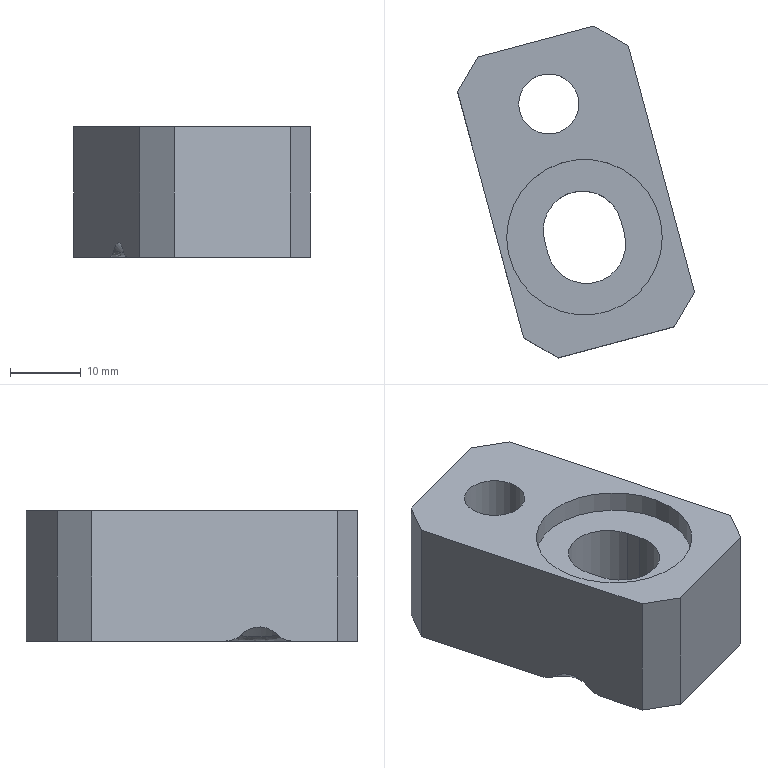Part | NX | features solid 2 | 1 solid | 21 faces | box 33.466 x 46.901 x 18.4 mm | volume 14639 mm3 | plane 14 | cylinder 6 | spline 1 | commonest cylinder face diameters 11.15 x2 8.5 x1 10 x1 14 x1 22 x1
STEP:
#1=CARTESIAN_POINT('',(1426.059,51.189,5.));
#2=VERTEX_POINT('',#1);
#3=CARTESIAN_POINT('',(1421.809,51.189,5.));
#4=DIRECTION('',(0.,0.,1.));
#5=DIRECTION('',(1.,0.,0.));
#6=AXIS2_PLACEMENT_3D('',#3,#4,#5);
#7=CIRCLE('',#6,4.25);
#8=EDGE_CURVE('',#2,#2,#7,.T.);
#9=ORIENTED_EDGE('',*,*,#8,.F.);
#10=EDGE_LOOP('',(#9));
#11=FACE_BOUND('',#10,.T.);
#12=CARTESIAN_POINT('',(1408.924,52.912,5.));
#13=VERTEX_POINT('',#12);
#14=CARTESIAN_POINT('',(1418.241,18.139,5.));
#15=VERTEX_POINT('',#14);
#16=CARTESIAN_POINT('',(1407.889,56.776,5.));
#17=DIRECTION('',(0.2588,-0.9659,0.));
#18=VECTOR('',#17,1000.);
#19=LINE('',#16,#18);
#20=EDGE_CURVE('',#13,#15,#19,.T.);
#21=ORIENTED_EDGE('',*,*,#20,.T.);
#22=CARTESIAN_POINT('',(1423.14,15.311,5.));
#23=VERTEX_POINT('',#22);
#24=CARTESIAN_POINT('',(362.415,627.721,5.));
#25=DIRECTION('',(0.866,-0.5,0.));
#26=VECTOR('',#25,1000.);
#27=LINE('',#24,#26);
#28=EDGE_CURVE('',#15,#23,#27,.T.);
#29=ORIENTED_EDGE('',*,*,#28,.T.);
#30=CARTESIAN_POINT('',(1439.561,19.711,5.));
#31=VERTEX_POINT('',#30);
#32=CARTESIAN_POINT('',(1419.277,14.275,5.));
#33=DIRECTION('',(0.9659,0.2588,0.));
#34=VECTOR('',#33,1000.);
#35=LINE('',#32,#34);
#36=EDGE_CURVE('',#23,#31,#35,.T.);
#37=ORIENTED_EDGE('',*,*,#36,.T.);
#38=CARTESIAN_POINT('',(1442.39,24.61,5.));
#39=VERTEX_POINT('',#38);
#40=CARTESIAN_POINT('',(1071.136,-618.421,5.));
#41=DIRECTION('',(0.5,0.866,0.));
#42=VECTOR('',#41,1000.);
#43=LINE('',#40,#42);
#44=EDGE_CURVE('',#31,#39,#43,.T.);
#45=ORIENTED_EDGE('',*,*,#44,.T.);
#46=CARTESIAN_POINT('',(1433.072,59.383,5.));
#47=VERTEX_POINT('',#46);
#48=CARTESIAN_POINT('',(1443.425,20.746,5.));
#49=DIRECTION('',(-0.2588,0.9659,0.));
#50=VECTOR('',#49,1000.);
#51=LINE('',#48,#50);
#52=EDGE_CURVE('',#39,#47,#51,.T.);
#53=ORIENTED_EDGE('',*,*,#52,.T.);
#54=CARTESIAN_POINT('',(1428.173,62.211,5.));
#55=VERTEX_POINT('',#54);
#56=CARTESIAN_POINT('',(383.982,665.076,5.));
#57=DIRECTION('',(0.866,-0.5,0.));
#58=VECTOR('',#57,1000.);
#59=LINE('',#56,#58);
#60=EDGE_CURVE('',#47,#55,#59,.F.);
#61=ORIENTED_EDGE('',*,*,#60,.T.);
#62=CARTESIAN_POINT('',(1411.752,57.811,5.));
#63=VERTEX_POINT('',#62);
#64=CARTESIAN_POINT('',(1432.037,63.247,5.));
#65=DIRECTION('',(-0.9659,-0.2588,0.));
#66=VECTOR('',#65,1000.);
#67=LINE('',#64,#66);
#68=EDGE_CURVE('',#55,#63,#67,.T.);
#69=ORIENTED_EDGE('',*,*,#68,.T.);
#70=CARTESIAN_POINT('',(1033.781,-596.854,5.));
#71=DIRECTION('',(0.5,0.866,0.));
#72=VECTOR('',#71,1000.);
#73=LINE('',#70,#72);
#74=EDGE_CURVE('',#63,#13,#73,.F.);
#75=ORIENTED_EDGE('',*,*,#74,.T.);
#76=EDGE_LOOP('',(#21,#29,#37,#45,#53,#61,#69,#75));
#77=FACE_BOUND('',#76,.T.);
#78=CARTESIAN_POINT('',(1437.856,32.353,5.));
#79=VERTEX_POINT('',#78);
#80=CARTESIAN_POINT('',(1426.856,32.353,5.));
#81=DIRECTION('',(0.,0.,1.));
#82=DIRECTION('',(1.,0.,0.));
#83=AXIS2_PLACEMENT_3D('',#80,#81,#82);
#84=CIRCLE('',#83,11.);
#85=EDGE_CURVE('',#79,#79,#84,.F.);
#86=ORIENTED_EDGE('',*,*,#85,.T.);
#87=EDGE_LOOP('',(#86));
#88=FACE_BOUND('',#87,.T.);
#89=CARTESIAN_POINT('',(0.,0.,5.));
#90=DIRECTION('',(0.,0.,1.));
#91=DIRECTION('',(1.,0.,0.));
#92=AXIS2_PLACEMENT_3D('',#89,#90,#91);
#93=PLANE('',#92);
#94=ADVANCED_FACE('',(#11,#77,#88),#93,.T.);
#95=ORIENTED_EDGE('',*,*,#85,.F.);
#96=EDGE_LOOP('',(#95));
#97=FACE_BOUND('',#96,.T.);
#98=CARTESIAN_POINT('',(1415.856,32.353,2.));
#99=VERTEX_POINT('',#98);
#100=CARTESIAN_POINT('',(1426.856,32.353,2.));
#101=DIRECTION('',(0.,0.,1.));
#102=DIRECTION('',(-1.,0.,0.));
#103=AXIS2_PLACEMENT_3D('',#100,#101,#102);
#104=CIRCLE('',#103,11.);
#105=EDGE_CURVE('',#99,#99,#104,.T.);
#106=ORIENTED_EDGE('',*,*,#105,.F.);
#107=EDGE_LOOP('',(#106));
#108=FACE_BOUND('',#107,.T.);
#109=CARTESIAN_POINT('',(1426.856,32.353,258.));
#110=DIRECTION('',(0.,0.,-1.));
#111=DIRECTION('',(-1.,0.,0.));
#112=AXIS2_PLACEMENT_3D('',#109,#110,#111);
#113=CYLINDRICAL_SURFACE('',#112,11.);
#114=ADVANCED_FACE('',(#97,#108),#113,.F.);
#115=CARTESIAN_POINT('',(1431.982,34.762,2.));
#116=VERTEX_POINT('',#115);
#117=CARTESIAN_POINT('',(1431.982,34.762,-13.4));
#118=VERTEX_POINT('',#117);
#119=CARTESIAN_POINT('',(1431.982,34.762,-16.4));
#120=DIRECTION('',(0.,0.,1.));
#121=VECTOR('',#120,1000.);
#122=LINE('',#119,#121);
#123=EDGE_CURVE('',#116,#118,#122,.F.);
#124=ORIENTED_EDGE('',*,*,#123,.T.);
#125=CARTESIAN_POINT('',(1432.5,32.83,-13.4));
#126=VERTEX_POINT('',#125);
#127=CARTESIAN_POINT('',(1429.265,44.904,-13.4));
#128=DIRECTION('',(-0.2588,0.9659,0.));
#129=VECTOR('',#128,1000.);
#130=LINE('',#127,#129);
#131=EDGE_CURVE('',#118,#126,#130,.F.);
#132=ORIENTED_EDGE('',*,*,#131,.T.);
#133=CARTESIAN_POINT('',(1432.5,32.83,2.));
#134=VERTEX_POINT('',#133);
#135=CARTESIAN_POINT('',(1432.5,32.83,-16.4));
#136=DIRECTION('',(0.,0.,1.));
#137=VECTOR('',#136,1000.);
#138=LINE('',#135,#137);
#139=EDGE_CURVE('',#134,#126,#138,.F.);
#140=ORIENTED_EDGE('',*,*,#139,.F.);
#141=CARTESIAN_POINT('',(1429.265,44.904,2.));
#142=DIRECTION('',(-0.2588,0.9659,0.));
#143=VECTOR('',#142,1000.);
#144=LINE('',#141,#143);
#145=EDGE_CURVE('',#116,#134,#144,.F.);
#146=ORIENTED_EDGE('',*,*,#145,.F.);
#147=EDGE_LOOP('',(#124,#132,#140,#146));
#148=FACE_BOUND('',#147,.T.);
#149=CARTESIAN_POINT('',(1429.265,44.904,-16.4));
#150=DIRECTION('',(-0.9659,-0.2588,0.));
#151=DIRECTION('',(0.2588,-0.9659,0.));
#152=AXIS2_PLACEMENT_3D('',#149,#150,#151);
#153=PLANE('',#152);
#154=ADVANCED_FACE('',(#148),#153,.T.);
#155=ORIENTED_EDGE('',*,*,#139,.T.);
#156=CARTESIAN_POINT('',(1421.73,29.944,-13.4));
#157=VERTEX_POINT('',#156);
#158=CARTESIAN_POINT('',(1427.115,31.387,-13.4));
#159=DIRECTION('',(0.,0.,1.));
#160=DIRECTION('',(1.,0.,0.));
#161=AXIS2_PLACEMENT_3D('',#158,#159,#160);
#162=CIRCLE('',#161,5.575);
#163=EDGE_CURVE('',#126,#157,#162,.F.);
#164=ORIENTED_EDGE('',*,*,#163,.T.);
#165=CARTESIAN_POINT('',(1421.73,29.944,2.));
#166=VERTEX_POINT('',#165);
#167=CARTESIAN_POINT('',(1421.73,29.944,-16.4));
#168=DIRECTION('',(0.,0.,1.));
#169=VECTOR('',#168,1000.);
#170=LINE('',#167,#169);
#171=EDGE_CURVE('',#166,#157,#170,.F.);
#172=ORIENTED_EDGE('',*,*,#171,.F.);
#173=CARTESIAN_POINT('',(1427.115,31.387,2.));
#174=DIRECTION('',(0.,0.,1.));
#175=DIRECTION('',(-1.,0.,0.));
#176=AXIS2_PLACEMENT_3D('',#173,#174,#175);
#177=CIRCLE('',#176,5.575);
#178=EDGE_CURVE('',#166,#134,#177,.T.);
#179=ORIENTED_EDGE('',*,*,#178,.T.);
#180=EDGE_LOOP('',(#155,#164,#172,#179));
#181=FACE_BOUND('',#180,.T.);
#182=CARTESIAN_POINT('',(1427.115,31.387,-16.4));
#183=DIRECTION('',(0.,0.,1.));
#184=DIRECTION('',(1.,0.,0.));
#185=AXIS2_PLACEMENT_3D('',#182,#183,#184);
#186=CYLINDRICAL_SURFACE('',#185,5.575);
#187=ADVANCED_FACE('',(#181),#186,.F.);
#188=ORIENTED_EDGE('',*,*,#171,.T.);
#189=CARTESIAN_POINT('',(1421.212,31.876,-13.4));
#190=VERTEX_POINT('',#189);
#191=CARTESIAN_POINT('',(1418.495,42.018,-13.4));
#192=DIRECTION('',(0.2588,-0.9659,0.));
#193=VECTOR('',#192,1000.);
#194=LINE('',#191,#193);
#195=EDGE_CURVE('',#157,#190,#194,.F.);
#196=ORIENTED_EDGE('',*,*,#195,.T.);
#197=CARTESIAN_POINT('',(1421.212,31.876,2.));
#198=VERTEX_POINT('',#197);
#199=CARTESIAN_POINT('',(1421.212,31.876,-16.4));
#200=DIRECTION('',(0.,0.,1.));
#201=VECTOR('',#200,1000.);
#202=LINE('',#199,#201);
#203=EDGE_CURVE('',#198,#190,#202,.F.);
#204=ORIENTED_EDGE('',*,*,#203,.F.);
#205=CARTESIAN_POINT('',(1418.495,42.018,2.));
#206=DIRECTION('',(0.2588,-0.9659,0.));
#207=VECTOR('',#206,1000.);
#208=LINE('',#205,#207);
#209=EDGE_CURVE('',#166,#198,#208,.F.);
#210=ORIENTED_EDGE('',*,*,#209,.F.);
#211=EDGE_LOOP('',(#188,#196,#204,#210));
#212=FACE_BOUND('',#211,.T.);
#213=CARTESIAN_POINT('',(1418.495,42.018,-16.4));
#214=DIRECTION('',(0.9659,0.2588,0.));
#215=DIRECTION('',(-0.2588,0.9659,0.));
#216=AXIS2_PLACEMENT_3D('',#213,#214,#215);
#217=PLANE('',#216);
#218=ADVANCED_FACE('',(#212),#217,.T.);
#219=CARTESIAN_POINT('',(1433.072,59.383,-13.4));
#220=VERTEX_POINT('',#219);
#221=CARTESIAN_POINT('',(1442.39,24.61,-13.4));
#222=VERTEX_POINT('',#221);
#223=CARTESIAN_POINT('',(1436.437,46.826,-13.4));
#224=DIRECTION('',(-0.2588,0.9659,0.));
#225=VECTOR('',#224,1000.);
#226=LINE('',#223,#225);
#227=EDGE_CURVE('',#220,#222,#226,.F.);
#228=ORIENTED_EDGE('',*,*,#227,.F.);
#229=CARTESIAN_POINT('',(1433.072,59.383,-16.4));
#230=DIRECTION('',(0.,0.,-1.));
#231=VECTOR('',#230,1000.);
#232=LINE('',#229,#231);
#233=EDGE_CURVE('',#220,#47,#232,.F.);
#234=ORIENTED_EDGE('',*,*,#233,.T.);
#235=ORIENTED_EDGE('',*,*,#52,.F.);
#236=CARTESIAN_POINT('',(1442.39,24.61,-16.4));
#237=DIRECTION('',(0.,0.,1.));
#238=VECTOR('',#237,1000.);
#239=LINE('',#236,#238);
#240=EDGE_CURVE('',#39,#222,#239,.F.);
#241=ORIENTED_EDGE('',*,*,#240,.T.);
#242=EDGE_LOOP('',(#228,#234,#235,#241));
#243=FACE_BOUND('',#242,.T.);
#244=CARTESIAN_POINT('',(1436.437,46.826,-16.4));
#245=DIRECTION('',(0.9659,0.2588,0.));
#246=DIRECTION('',(-0.2588,0.9659,0.));
#247=AXIS2_PLACEMENT_3D('',#244,#245,#246);
#248=PLANE('',#247);
#249=ADVANCED_FACE('',(#243),#248,.T.);
#250=CARTESIAN_POINT('',(1411.752,57.811,-13.4));
#251=VERTEX_POINT('',#250);
#252=CARTESIAN_POINT('',(1428.173,62.211,-13.4));
#253=VERTEX_POINT('',#252);
#254=CARTESIAN_POINT('',(1405.957,56.258,-13.4));
#255=DIRECTION('',(-0.9659,-0.2588,0.));
#256=VECTOR('',#255,1000.);
#257=LINE('',#254,#256);
#258=EDGE_CURVE('',#251,#253,#257,.F.);
#259=ORIENTED_EDGE('',*,*,#258,.F.);
#260=CARTESIAN_POINT('',(1411.752,57.811,-16.4));
#261=DIRECTION('',(0.,0.,-1.));
#262=VECTOR('',#261,1000.);
#263=LINE('',#260,#262);
#264=EDGE_CURVE('',#251,#63,#263,.F.);
#265=ORIENTED_EDGE('',*,*,#264,.T.);
#266=ORIENTED_EDGE('',*,*,#68,.F.);
#267=CARTESIAN_POINT('',(1428.173,62.211,-16.4));
#268=DIRECTION('',(0.,0.,1.));
#269=VECTOR('',#268,1000.);
#270=LINE('',#267,#269);
#271=EDGE_CURVE('',#55,#253,#270,.F.);
#272=ORIENTED_EDGE('',*,*,#271,.T.);
#273=EDGE_LOOP('',(#259,#265,#266,#272));
#274=FACE_BOUND('',#273,.T.);
#275=CARTESIAN_POINT('',(1405.957,56.258,-16.4));
#276=DIRECTION('',(-0.2588,0.9659,0.));
#277=DIRECTION('',(-0.9659,-0.2588,0.));
#278=AXIS2_PLACEMENT_3D('',#275,#276,#277);
#279=PLANE('',#278);
#280=ADVANCED_FACE('',(#274),#279,.T.);
#281=CARTESIAN_POINT('',(1416.533,24.515,-13.4));
#282=VERTEX_POINT('',#281);
#283=CARTESIAN_POINT('',(1418.241,18.139,-13.4));
#284=VERTEX_POINT('',#283);
#285=CARTESIAN_POINT('',(1413.255,36.748,-13.4));
#286=DIRECTION('',(-0.2588,0.9659,0.));
#287=VECTOR('',#286,1000.);
#288=LINE('',#285,#287);
#289=EDGE_CURVE('',#282,#284,#288,.F.);
#290=ORIENTED_EDGE('',*,*,#289,.T.);
#291=CARTESIAN_POINT('',(1418.241,18.139,-16.4));
#292=DIRECTION('',(0.,0.,-1.));
#293=VECTOR('',#292,1000.);
#294=LINE('',#291,#293);
#295=EDGE_CURVE('',#284,#15,#294,.F.);
#296=ORIENTED_EDGE('',*,*,#295,.T.);
#297=ORIENTED_EDGE('',*,*,#20,.F.);
#298=CARTESIAN_POINT('',(1408.924,52.912,-13.4));
#299=VERTEX_POINT('',#298);
#300=CARTESIAN_POINT('',(1408.924,52.912,-16.4));
#301=DIRECTION('',(0.,0.,1.));
#302=VECTOR('',#301,1000.);
#303=LINE('',#300,#302);
#304=EDGE_CURVE('',#13,#299,#303,.F.);
#305=ORIENTED_EDGE('',*,*,#304,.T.);
#306=CARTESIAN_POINT('',(1413.997,33.979,-13.4));
#307=VERTEX_POINT('',#306);
#308=CARTESIAN_POINT('',(1413.255,36.748,-13.4));
#309=DIRECTION('',(-0.2588,0.9659,0.));
#310=VECTOR('',#309,1000.);
#311=LINE('',#308,#310);
#312=EDGE_CURVE('',#299,#307,#311,.F.);
#313=ORIENTED_EDGE('',*,*,#312,.T.);
#314=CARTESIAN_POINT('',(1414.55,31.917,-12.578));
#315=VERTEX_POINT('',#314);
#316=CARTESIAN_POINT('',(1413.997,33.979,-13.4));
#317=CARTESIAN_POINT('',(1414.201,33.219,-13.4));
#318=CARTESIAN_POINT('',(1414.401,32.472,-13.117));
#319=CARTESIAN_POINT('',(1414.55,31.917,-12.579));
#320=B_SPLINE_CURVE_WITH_KNOTS('',3,(#316,#317,#318,#319),.UNSPECIFIED.,.F.,.F.,(4,4),(0.,0.002329),.UNSPECIFIED.);
#321=EDGE_CURVE('',#307,#315,#320,.T.);
#322=ORIENTED_EDGE('',*,*,#321,.T.);
#323=CARTESIAN_POINT('',(1415.98,26.578,-12.578));
#324=VERTEX_POINT('',#323);
#325=CARTESIAN_POINT('',(1415.265,29.247,-18.471));
#326=DIRECTION('',(-0.9659,-0.2588,0.));
#327=DIRECTION('',(0.,0.,1.));
#328=AXIS2_PLACEMENT_3D('',#325,#326,#327);
#329=ELLIPSE('',#328,7.071,5.);
#330=EDGE_CURVE('',#315,#324,#329,.F.);
#331=ORIENTED_EDGE('',*,*,#330,.T.);
#332=CARTESIAN_POINT('',(1415.98,26.578,-12.579));
#333=CARTESIAN_POINT('',(1416.129,26.023,-13.117));
#334=CARTESIAN_POINT('',(1416.33,25.274,-13.4));
#335=CARTESIAN_POINT('',(1416.533,24.515,-13.4));
#336=B_SPLINE_CURVE_WITH_KNOTS('',3,(#332,#333,#334,#335),.UNSPECIFIED.,.F.,.F.,(4,4),(0.,0.002325),.UNSPECIFIED.);
#337=EDGE_CURVE('',#324,#282,#336,.T.);
#338=ORIENTED_EDGE('',*,*,#337,.T.);
#339=EDGE_LOOP('',(#290,#296,#297,#305,#313,#322,#331,#338));
#340=FACE_BOUND('',#339,.T.);
#341=CARTESIAN_POINT('',(1413.255,36.748,-16.4));
#342=DIRECTION('',(-0.9659,-0.2588,0.));
#343=DIRECTION('',(0.2588,-0.9659,0.));
#344=AXIS2_PLACEMENT_3D('',#341,#342,#343);
#345=PLANE('',#344);
#346=ADVANCED_FACE('',(#340),#345,.T.);
#347=ORIENTED_EDGE('',*,*,#36,.F.);
#348=CARTESIAN_POINT('',(1423.14,15.311,-13.4));
#349=VERTEX_POINT('',#348);
#350=CARTESIAN_POINT('',(1423.14,15.311,-16.4));
#351=DIRECTION('',(0.,0.,-1.));
#352=VECTOR('',#351,1000.);
#353=LINE('',#350,#352);
#354=EDGE_CURVE('',#23,#349,#353,.T.);
#355=ORIENTED_EDGE('',*,*,#354,.T.);
#356=CARTESIAN_POINT('',(1439.561,19.711,-13.4));
#357=VERTEX_POINT('',#356);
#358=CARTESIAN_POINT('',(1417.345,13.758,-13.4));
#359=DIRECTION('',(0.9659,0.2588,0.));
#360=VECTOR('',#359,1000.);
#361=LINE('',#358,#360);
#362=EDGE_CURVE('',#349,#357,#361,.T.);
#363=ORIENTED_EDGE('',*,*,#362,.T.);
#364=CARTESIAN_POINT('',(1439.561,19.711,-16.4));
#365=DIRECTION('',(0.,0.,1.));
#366=VECTOR('',#365,1000.);
#367=LINE('',#364,#366);
#368=EDGE_CURVE('',#357,#31,#367,.T.);
#369=ORIENTED_EDGE('',*,*,#368,.T.);
#370=EDGE_LOOP('',(#347,#355,#363,#369));
#371=FACE_BOUND('',#370,.T.);
#372=CARTESIAN_POINT('',(1417.345,13.758,-16.4));
#373=DIRECTION('',(-0.2588,0.9659,0.));
#374=DIRECTION('',(-0.9659,-0.2588,0.));
#375=AXIS2_PLACEMENT_3D('',#372,#373,#374);
#376=PLANE('',#375);
#377=ADVANCED_FACE('',(#371),#376,.F.);
#378=ORIENTED_EDGE('',*,*,#203,.T.);
#379=CARTESIAN_POINT('',(1426.597,33.319,-13.4));
#380=DIRECTION('',(0.,0.,1.));
#381=DIRECTION('',(1.,0.,0.));
#382=AXIS2_PLACEMENT_3D('',#379,#380,#381);
#383=CIRCLE('',#382,5.575);
#384=EDGE_CURVE('',#190,#118,#383,.F.);
#385=ORIENTED_EDGE('',*,*,#384,.T.);
#386=ORIENTED_EDGE('',*,*,#123,.F.);
#387=CARTESIAN_POINT('',(1426.597,33.319,2.));
#388=DIRECTION('',(0.,0.,1.));
#389=DIRECTION('',(-1.,0.,0.));
#390=AXIS2_PLACEMENT_3D('',#387,#388,#389);
#391=CIRCLE('',#390,5.575);
#392=EDGE_CURVE('',#116,#198,#391,.T.);
#393=ORIENTED_EDGE('',*,*,#392,.T.);
#394=EDGE_LOOP('',(#378,#385,#386,#393));
#395=FACE_BOUND('',#394,.T.);
#396=CARTESIAN_POINT('',(1426.597,33.319,-16.4));
#397=DIRECTION('',(0.,0.,1.));
#398=DIRECTION('',(1.,0.,0.));
#399=AXIS2_PLACEMENT_3D('',#396,#397,#398);
#400=CYLINDRICAL_SURFACE('',#399,5.575);
#401=ADVANCED_FACE('',(#395),#400,.F.);
#402=CARTESIAN_POINT('',(1428.809,51.189,-13.4));
#403=VERTEX_POINT('',#402);
#404=CARTESIAN_POINT('',(1421.809,51.189,-13.4));
#405=DIRECTION('',(0.,0.,1.));
#406=DIRECTION('',(1.,0.,0.));
#407=AXIS2_PLACEMENT_3D('',#404,#405,#406);
#408=CIRCLE('',#407,7.);
#409=EDGE_CURVE('',#403,#403,#408,.T.);
#410=ORIENTED_EDGE('',*,*,#409,.T.);
#411=EDGE_LOOP('',(#410));
#412=FACE_BOUND('',#411,.T.);
#413=ORIENTED_EDGE('',*,*,#362,.F.);
#414=CARTESIAN_POINT('',(1418.241,18.139,-13.4));
#415=DIRECTION('',(-0.866,0.5,0.));
#416=VECTOR('',#415,1000.);
#417=LINE('',#414,#416);
#418=EDGE_CURVE('',#349,#284,#417,.T.);
#419=ORIENTED_EDGE('',*,*,#418,.T.);
#420=ORIENTED_EDGE('',*,*,#289,.F.);
#421=CARTESIAN_POINT('',(1413.997,33.979,-13.4));
#422=CARTESIAN_POINT('',(1414.228,33.891,-13.4));
#423=CARTESIAN_POINT('',(1414.564,33.748,-13.4));
#424=CARTESIAN_POINT('',(1414.934,33.559,-13.4));
#425=CARTESIAN_POINT('',(1415.115,33.46,-13.4));
#426=CARTESIAN_POINT('',(1415.204,33.409,-13.4));
#427=CARTESIAN_POINT('',(1415.241,33.387,-13.4));
#428=CARTESIAN_POINT('',(1415.266,33.372,-13.4));
#429=CARTESIAN_POINT('',(1415.278,33.365,-13.4));
#430=CARTESIAN_POINT('',(1415.508,33.228,-13.4));
#431=CARTESIAN_POINT('',(1415.815,33.022,-13.4));
#432=CARTESIAN_POINT('',(1416.146,32.761,-13.4));
#433=CARTESIAN_POINT('',(1416.304,32.625,-13.4));
#434=CARTESIAN_POINT('',(1416.381,32.556,-13.4));
#435=CARTESIAN_POINT('',(1416.414,32.526,-13.4));
#436=CARTESIAN_POINT('',(1416.436,32.506,-13.4));
#437=CARTESIAN_POINT('',(1416.446,32.497,-13.4));
#438=CARTESIAN_POINT('',(1416.643,32.312,-13.4));
#439=CARTESIAN_POINT('',(1416.901,32.039,-13.4));
#440=CARTESIAN_POINT('',(1417.163,31.7,-13.4));
#441=CARTESIAN_POINT('',(1417.284,31.526,-13.4));
#442=CARTESIAN_POINT('',(1417.335,31.45,-13.4));
#443=CARTESIAN_POINT('',(1417.367,31.399,-13.4));
#444=CARTESIAN_POINT('',(1417.383,31.375,-13.4));
#445=CARTESIAN_POINT('',(1417.669,30.917,-13.4));
#446=CARTESIAN_POINT('',(1417.868,30.46,-13.4));
#447=CARTESIAN_POINT('',(1418.061,29.739,-13.4));
#448=CARTESIAN_POINT('',(1418.131,29.374,-13.4));
#449=CARTESIAN_POINT('',(1418.163,28.938,-13.4));
#450=CARTESIAN_POINT('',(1418.168,28.717,-13.4));
#451=CARTESIAN_POINT('',(1418.167,28.623,-13.4));
#452=CARTESIAN_POINT('',(1418.166,28.559,-13.4));
#453=CARTESIAN_POINT('',(1418.165,28.526,-13.4));
#454=CARTESIAN_POINT('',(1418.156,28.254,-13.4));
#455=CARTESIAN_POINT('',(1418.119,27.891,-13.4));
#456=CARTESIAN_POINT('',(1418.032,27.466,-13.4));
#457=CARTESIAN_POINT('',(1417.978,27.252,-13.4));
#458=CARTESIAN_POINT('',(1417.948,27.146,-13.4));
#459=CARTESIAN_POINT('',(1417.935,27.1,-13.4));
#460=CARTESIAN_POINT('',(1417.926,27.069,-13.4));
#461=CARTESIAN_POINT('',(1417.921,27.053,-13.4));
#462=CARTESIAN_POINT('',(1417.848,26.813,-13.4));
#463=CARTESIAN_POINT('',(1417.725,26.476,-13.4));
#464=CARTESIAN_POINT('',(1417.546,26.087,-13.4));
#465=CARTESIAN_POINT('',(1417.447,25.894,-13.4));
#466=CARTESIAN_POINT('',(1417.396,25.797,-13.4));
#467=CARTESIAN_POINT('',(1417.373,25.756,-13.4));
#468=CARTESIAN_POINT('',(1417.358,25.728,-13.4));
#469=CARTESIAN_POINT('',(1417.35,25.713,-13.4));
#470=CARTESIAN_POINT('',(1417.116,25.294,-13.4));
#471=CARTESIAN_POINT('',(1416.846,24.899,-13.4));
#472=CARTESIAN_POINT('',(1416.533,24.515,-13.4));
#473=B_SPLINE_CURVE_WITH_KNOTS('',3,(#421,#422,#423,#424,#425,#426,#427,#428,#429,#430,#431,#432,#433,#434,#435,#436,#437,#438,#439,#440,#441,#442,#443,#444,#445,#446,#447,#448,#449,#450,#451,#452,#453,#454,#455,#456,#457,#458,#459,#460,#461,#462,#463,#464,#465,#466,#467,#468,#469,#470,#471,#472),.UNSPECIFIED.,.F.,.F.,(4,1,1,1,1,2,2,1,1,1,1,2,2,1,1,1,2,2,2,1,1,1,2,2,1,1,1,1,2,2,1,1,1,1,2,2,4),(0.,0.0625,0.09375,0.1094,0.1172,0.1211,0.125,0.1875,0.2187,0.2344,0.2422,0.2461,0.25,0.3125,0.3437,0.3594,0.3672,0.375,0.5,0.5625,0.5937,0.6094,0.6172,0.625,0.6875,0.7187,0.7344,0.7422,0.7461,0.75,0.8125,0.8437,0.8594,0.8672,0.8711,0.875,1.),.UNSPECIFIED.);
#474=EDGE_CURVE('',#307,#282,#473,.T.);
#475=ORIENTED_EDGE('',*,*,#474,.F.);
#476=ORIENTED_EDGE('',*,*,#312,.F.);
#477=CARTESIAN_POINT('',(1411.752,57.811,-13.4));
#478=DIRECTION('',(-0.5,-0.866,0.));
#479=VECTOR('',#478,1000.);
#480=LINE('',#477,#479);
#481=EDGE_CURVE('',#299,#251,#480,.F.);
#482=ORIENTED_EDGE('',*,*,#481,.T.);
#483=ORIENTED_EDGE('',*,*,#258,.T.);
#484=CARTESIAN_POINT('',(1433.072,59.383,-13.4));
#485=DIRECTION('',(-0.866,0.5,0.));
#486=VECTOR('',#485,1000.);
#487=LINE('',#484,#486);
#488=EDGE_CURVE('',#253,#220,#487,.F.);
#489=ORIENTED_EDGE('',*,*,#488,.T.);
#490=ORIENTED_EDGE('',*,*,#227,.T.);
#491=CARTESIAN_POINT('',(1439.561,19.711,-13.4));
#492=DIRECTION('',(-0.5,-0.866,0.));
#493=VECTOR('',#492,1000.);
#494=LINE('',#491,#493);
#495=EDGE_CURVE('',#222,#357,#494,.T.);
#496=ORIENTED_EDGE('',*,*,#495,.T.);
#497=EDGE_LOOP('',(#413,#419,#420,#475,#476,#482,#483,#489,#490,#496));
#498=FACE_BOUND('',#497,.T.);
#499=ORIENTED_EDGE('',*,*,#195,.F.);
#500=ORIENTED_EDGE('',*,*,#163,.F.);
#501=ORIENTED_EDGE('',*,*,#131,.F.);
#502=ORIENTED_EDGE('',*,*,#384,.F.);
#503=EDGE_LOOP('',(#499,#500,#501,#502));
#504=FACE_BOUND('',#503,.T.);
#505=CARTESIAN_POINT('',(1410.357,39.838,-13.4));
#506=DIRECTION('',(0.,0.,1.));
#507=DIRECTION('',(-0.2588,0.9659,0.));
#508=AXIS2_PLACEMENT_3D('',#505,#506,#507);
#509=PLANE('',#508);
#510=ADVANCED_FACE('',(#412,#498,#504),#509,.F.);
#511=CARTESIAN_POINT('',(1416.631,29.613,-12.814));
#512=VERTEX_POINT('',#511);
#513=CARTESIAN_POINT('',(1416.631,29.613,-12.814));
#514=CARTESIAN_POINT('',(1416.5,30.101,-12.814));
#515=CARTESIAN_POINT('',(1416.105,30.8,-12.78));
#516=CARTESIAN_POINT('',(1415.232,31.538,-12.672));
#517=CARTESIAN_POINT('',(1414.8,31.791,-12.613));
#518=CARTESIAN_POINT('',(1414.55,31.917,-12.578));
#519=B_SPLINE_CURVE_WITH_KNOTS('',3,(#513,#514,#515,#516,#517,#518),.UNSPECIFIED.,.F.,.F.,(4,1,1,4),(0.,0.3712,0.5568,0.7424),.UNSPECIFIED.);
#520=EDGE_CURVE('',#315,#512,#519,.F.);
#521=ORIENTED_EDGE('',*,*,#520,.T.);
#522=CARTESIAN_POINT('',(1415.98,26.578,-12.578));
#523=CARTESIAN_POINT('',(1416.134,26.811,-12.613));
#524=CARTESIAN_POINT('',(1416.382,27.247,-12.672));
#525=CARTESIAN_POINT('',(1416.769,28.322,-12.78));
#526=CARTESIAN_POINT('',(1416.762,29.125,-12.814));
#527=CARTESIAN_POINT('',(1416.631,29.613,-12.814));
#528=B_SPLINE_CURVE_WITH_KNOTS('',3,(#522,#523,#524,#525,#526,#527),.UNSPECIFIED.,.F.,.F.,(4,1,1,4),(0.2576,0.4432,0.6288,1.),.UNSPECIFIED.);
#529=EDGE_CURVE('',#512,#324,#528,.F.);
#530=ORIENTED_EDGE('',*,*,#529,.T.);
#531=ORIENTED_EDGE('',*,*,#330,.F.);
#532=EDGE_LOOP('',(#521,#530,#531));
#533=FACE_BOUND('',#532,.T.);
#534=CARTESIAN_POINT('',(1411.815,28.323,-14.899));
#535=DIRECTION('',(-0.683,-0.183,0.7071));
#536=DIRECTION('',(-0.683,-0.183,-0.7071));
#537=AXIS2_PLACEMENT_3D('',#534,#535,#536);
#538=CYLINDRICAL_SURFACE('',#537,5.);
#539=ADVANCED_FACE('',(#533),#538,.F.);
#540=ORIENTED_EDGE('',*,*,#529,.F.);
#541=ORIENTED_EDGE('',*,*,#520,.F.);
#542=ORIENTED_EDGE('',*,*,#321,.F.);
#543=ORIENTED_EDGE('',*,*,#474,.T.);
#544=ORIENTED_EDGE('',*,*,#337,.F.);
#545=EDGE_LOOP('',(#540,#541,#542,#543,#544));
#546=FACE_BOUND('',#545,.T.);
#547=CARTESIAN_POINT('',(1413.384,32.366,-12.41));
#548=CARTESIAN_POINT('',(1413.509,32.696,-13.013));
#549=CARTESIAN_POINT('',(1413.753,33.338,-13.4));
#550=CARTESIAN_POINT('',(1414.002,33.991,-13.4));
#551=CARTESIAN_POINT('',(1414.126,32.152,-12.521));
#552=CARTESIAN_POINT('',(1414.293,32.485,-13.064));
#553=CARTESIAN_POINT('',(1414.591,33.065,-13.4));
#554=CARTESIAN_POINT('',(1414.893,33.651,-13.4));
#555=CARTESIAN_POINT('',(1414.833,31.832,-12.62));
#556=CARTESIAN_POINT('',(1415.047,32.147,-13.107));
#557=CARTESIAN_POINT('',(1415.396,32.654,-13.4));
#558=CARTESIAN_POINT('',(1415.748,33.165,-13.4));
#559=CARTESIAN_POINT('',(1415.998,30.913,-12.768));
#560=CARTESIAN_POINT('',(1416.299,31.148,-13.169));
#561=CARTESIAN_POINT('',(1416.739,31.484,-13.4));
#562=CARTESIAN_POINT('',(1417.181,31.822,-13.4));
#563=CARTESIAN_POINT('',(1416.446,30.305,-12.814));
#564=CARTESIAN_POINT('',(1416.786,30.474,-13.187));
#565=CARTESIAN_POINT('',(1417.265,30.712,-13.4));
#566=CARTESIAN_POINT('',(1417.747,30.952,-13.4));
#567=CARTESIAN_POINT('',(1416.816,28.922,-12.814));
#568=CARTESIAN_POINT('',(1417.196,28.946,-13.187));
#569=CARTESIAN_POINT('',(1417.73,28.979,-13.4));
#570=CARTESIAN_POINT('',(1418.266,29.013,-13.4));
#571=CARTESIAN_POINT('',(1416.733,28.171,-12.768));
#572=CARTESIAN_POINT('',(1417.111,28.119,-13.169));
#573=CARTESIAN_POINT('',(1417.66,28.047,-13.4));
#574=CARTESIAN_POINT('',(1418.212,27.976,-13.4));
#575=CARTESIAN_POINT('',(1416.183,26.793,-12.62));
#576=CARTESIAN_POINT('',(1416.526,26.627,-13.107));
#577=CARTESIAN_POINT('',(1417.082,26.362,-13.4));
#578=CARTESIAN_POINT('',(1417.642,26.096,-13.4));
#579=CARTESIAN_POINT('',(1415.732,26.162,-12.521));
#580=CARTESIAN_POINT('',(1416.042,25.957,-13.064));
#581=CARTESIAN_POINT('',(1416.59,25.604,-13.4));
#582=CARTESIAN_POINT('',(1417.145,25.247,-13.4));
#583=CARTESIAN_POINT('',(1415.195,25.606,-12.41));
#584=CARTESIAN_POINT('',(1415.468,25.383,-13.013));
#585=CARTESIAN_POINT('',(1416.002,24.948,-13.4));
#586=CARTESIAN_POINT('',(1416.543,24.507,-13.4));
#587=B_SPLINE_SURFACE_WITH_KNOTS('',3,3,((#547,#548,#549,#550),(#551,#552,#553,#554),(#555,#556,#557,#558),(#559,#560,#561,#562),(#563,#564,#565,#566),(#567,#568,#569,#570),(#571,#572,#573,#574),(#575,#576,#577,#578),(#579,#580,#581,#582),(#583,#584,#585,#586)),.UNSPECIFIED.,.F.,.F.,.F.,(4,2,2,2,4),(4,4),(0.,0.25,0.5,0.75,1.),(0.,1.006),.UNSPECIFIED.);
#588=ADVANCED_FACE('',(#546),#587,.F.);
#589=ORIENTED_EDGE('',*,*,#105,.T.);
#590=EDGE_LOOP('',(#589));
#591=FACE_BOUND('',#590,.T.);
#592=ORIENTED_EDGE('',*,*,#392,.F.);
#593=ORIENTED_EDGE('',*,*,#145,.T.);
#594=ORIENTED_EDGE('',*,*,#178,.F.);
#595=ORIENTED_EDGE('',*,*,#209,.T.);
#596=EDGE_LOOP('',(#592,#593,#594,#595));
#597=FACE_BOUND('',#596,.T.);
#598=CARTESIAN_POINT('',(1385.653,55.777,2.));
#599=DIRECTION('',(0.,0.,-1.));
#600=DIRECTION('',(-1.,0.,0.));
#601=AXIS2_PLACEMENT_3D('',#598,#599,#600);
#602=PLANE('',#601);
#603=ADVANCED_FACE('',(#591,#597),#602,.F.);
#604=ORIENTED_EDGE('',*,*,#8,.T.);
#605=EDGE_LOOP('',(#604));
#606=FACE_BOUND('',#605,.T.);
#607=CARTESIAN_POINT('',(1426.059,51.189,-3.4));
#608=VERTEX_POINT('',#607);
#609=CARTESIAN_POINT('',(1421.809,51.189,-3.4));
#610=DIRECTION('',(0.,0.,1.));
#611=DIRECTION('',(1.,0.,0.));
#612=AXIS2_PLACEMENT_3D('',#609,#610,#611);
#613=CIRCLE('',#612,4.25);
#614=EDGE_CURVE('',#608,#608,#613,.F.);
#615=ORIENTED_EDGE('',*,*,#614,.T.);
#616=EDGE_LOOP('',(#615));
#617=FACE_BOUND('',#616,.T.);
#618=CARTESIAN_POINT('',(1421.809,51.189,336.6));
#619=DIRECTION('',(0.,0.,1.));
#620=DIRECTION('',(1.,0.,0.));
#621=AXIS2_PLACEMENT_3D('',#618,#619,#620);
#622=CYLINDRICAL_SURFACE('',#621,4.25);
#623=ADVANCED_FACE('',(#606,#617),#622,.F.);
#624=ORIENTED_EDGE('',*,*,#614,.F.);
#625=EDGE_LOOP('',(#624));
#626=FACE_BOUND('',#625,.T.);
#627=CARTESIAN_POINT('',(1428.809,51.189,-3.4));
#628=VERTEX_POINT('',#627);
#629=CARTESIAN_POINT('',(1421.809,51.189,-3.4));
#630=DIRECTION('',(0.,0.,1.));
#631=DIRECTION('',(1.,0.,0.));
#632=AXIS2_PLACEMENT_3D('',#629,#630,#631);
#633=CIRCLE('',#632,7.);
#634=EDGE_CURVE('',#628,#628,#633,.F.);
#635=ORIENTED_EDGE('',*,*,#634,.T.);
#636=EDGE_LOOP('',(#635));
#637=FACE_BOUND('',#636,.T.);
#638=CARTESIAN_POINT('',(1420.85,52.952,-3.4));
#639=DIRECTION('',(0.,0.,1.));
#640=DIRECTION('',(1.,0.,0.));
#641=AXIS2_PLACEMENT_3D('',#638,#639,#640);
#642=PLANE('',#641);
#643=ADVANCED_FACE('',(#626,#637),#642,.F.);
#644=ORIENTED_EDGE('',*,*,#634,.F.);
#645=EDGE_LOOP('',(#644));
#646=FACE_BOUND('',#645,.T.);
#647=ORIENTED_EDGE('',*,*,#409,.F.);
#648=EDGE_LOOP('',(#647));
#649=FACE_BOUND('',#648,.T.);
#650=CARTESIAN_POINT('',(1421.809,51.189,-13.4));
#651=DIRECTION('',(0.,0.,1.));
#652=DIRECTION('',(1.,0.,0.));
#653=AXIS2_PLACEMENT_3D('',#650,#651,#652);
#654=CYLINDRICAL_SURFACE('',#653,7.);
#655=ADVANCED_FACE('',(#646,#649),#654,.F.);
#656=ORIENTED_EDGE('',*,*,#418,.F.);
#657=ORIENTED_EDGE('',*,*,#354,.F.);
#658=ORIENTED_EDGE('',*,*,#28,.F.);
#659=ORIENTED_EDGE('',*,*,#295,.F.);
#660=EDGE_LOOP('',(#656,#657,#658,#659));
#661=FACE_BOUND('',#660,.T.);
#662=CARTESIAN_POINT('',(1418.241,18.139,-16.4));
#663=DIRECTION('',(-0.5,-0.866,0.));
#664=DIRECTION('',(0.,0.,-1.));
#665=AXIS2_PLACEMENT_3D('',#662,#663,#664);
#666=PLANE('',#665);
#667=ADVANCED_FACE('',(#661),#666,.T.);
#668=ORIENTED_EDGE('',*,*,#481,.F.);
#669=ORIENTED_EDGE('',*,*,#304,.F.);
#670=ORIENTED_EDGE('',*,*,#74,.F.);
#671=ORIENTED_EDGE('',*,*,#264,.F.);
#672=EDGE_LOOP('',(#668,#669,#670,#671));
#673=FACE_BOUND('',#672,.T.);
#674=CARTESIAN_POINT('',(1411.752,57.811,-16.4));
#675=DIRECTION('',(0.866,-0.5,0.));
#676=DIRECTION('',(0.,0.,1.));
#677=AXIS2_PLACEMENT_3D('',#674,#675,#676);
#678=PLANE('',#677);
#679=ADVANCED_FACE('',(#673),#678,.F.);
#680=ORIENTED_EDGE('',*,*,#488,.F.);
#681=ORIENTED_EDGE('',*,*,#271,.F.);
#682=ORIENTED_EDGE('',*,*,#60,.F.);
#683=ORIENTED_EDGE('',*,*,#233,.F.);
#684=EDGE_LOOP('',(#680,#681,#682,#683));
#685=FACE_BOUND('',#684,.T.);
#686=CARTESIAN_POINT('',(1433.072,59.383,-16.4));
#687=DIRECTION('',(-0.5,-0.866,0.));
#688=DIRECTION('',(0.,0.,1.));
#689=AXIS2_PLACEMENT_3D('',#686,#687,#688);
#690=PLANE('',#689);
#691=ADVANCED_FACE('',(#685),#690,.F.);
#692=ORIENTED_EDGE('',*,*,#495,.F.);
#693=ORIENTED_EDGE('',*,*,#240,.F.);
#694=ORIENTED_EDGE('',*,*,#44,.F.);
#695=ORIENTED_EDGE('',*,*,#368,.F.);
#696=EDGE_LOOP('',(#692,#693,#694,#695));
#697=FACE_BOUND('',#696,.T.);
#698=CARTESIAN_POINT('',(1439.561,19.711,-16.4));
#699=DIRECTION('',(0.866,-0.5,0.));
#700=DIRECTION('',(0.,0.,-1.));
#701=AXIS2_PLACEMENT_3D('',#698,#699,#700);
#702=PLANE('',#701);
#703=ADVANCED_FACE('',(#697),#702,.T.);
#704=CLOSED_SHELL('',(#94,#114,#154,#187,#218,#249,#280,#346,#377,#401,#510,#539,#588,#603,#623,#643,#655,#667,#679,#691,#703));
#705=MANIFOLD_SOLID_BREP('',#704);
#706=(LENGTH_UNIT()NAMED_UNIT(*)SI_UNIT(.MILLI.,.METRE.));
#707=UNCERTAINTY_MEASURE_WITH_UNIT(LENGTH_MEASURE(0.0508),#706,'','');
#708=(NAMED_UNIT(*)PLANE_ANGLE_UNIT()SI_UNIT($,.RADIAN.));
#709=(NAMED_UNIT(*)SI_UNIT($,.STERADIAN.)SOLID_ANGLE_UNIT());
#710=(GEOMETRIC_REPRESENTATION_CONTEXT(3)GLOBAL_UNCERTAINTY_ASSIGNED_CONTEXT((#707))GLOBAL_UNIT_ASSIGNED_CONTEXT((#706,#708,#709))REPRESENTATION_CONTEXT('',''));
#711=ADVANCED_BREP_SHAPE_REPRESENTATION('',(#705),#710);